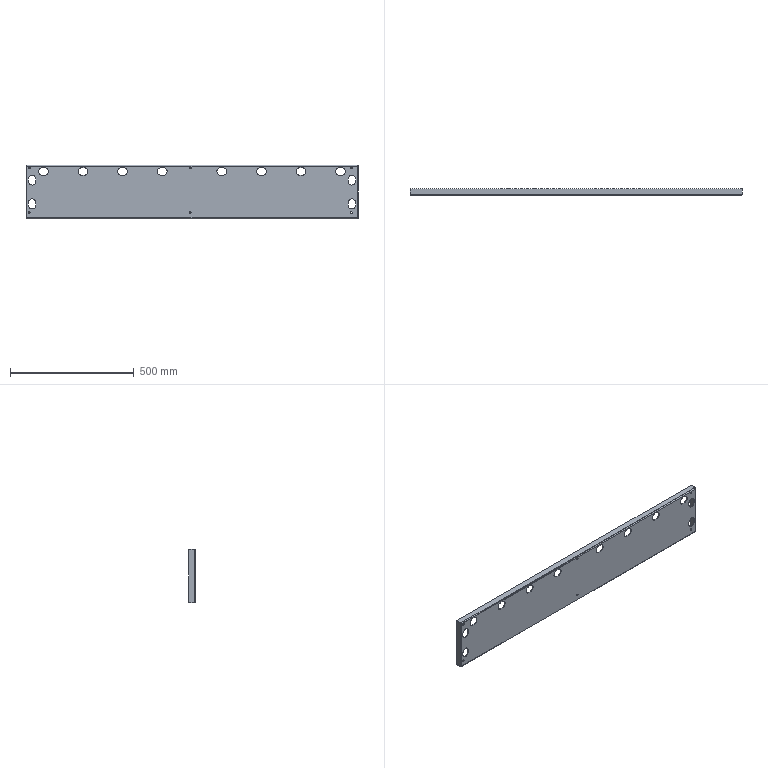Part | NX | features solid 2 | 1 solid | 110 faces | box 1340 x 27.5 x 216 mm | volume 704443 mm3 | plane 62 | cylinder 48 | commonest cylinder face diameters 30 x28 7.2 x12 4 x4 8 x4